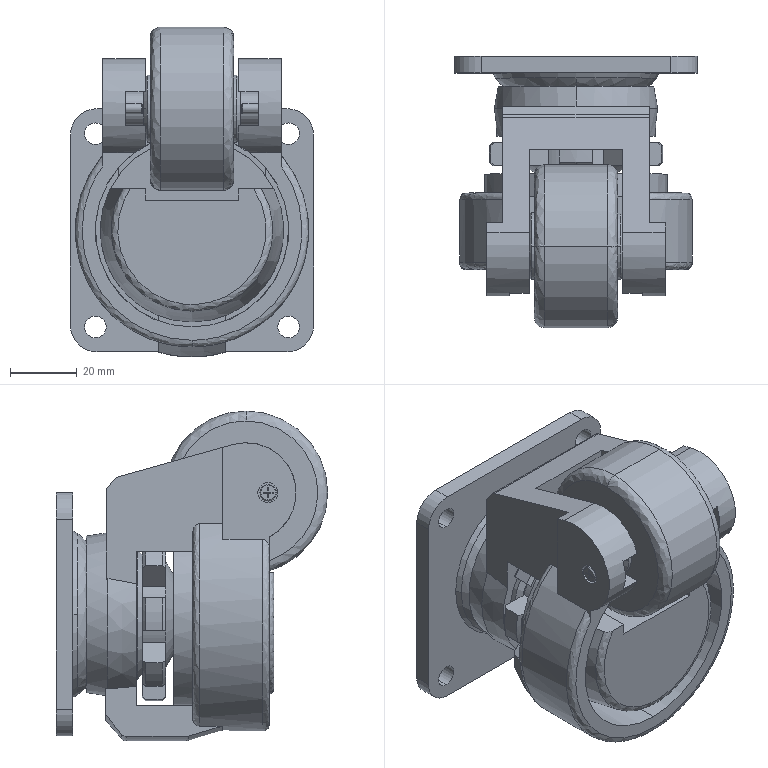Part | STEP file | CGR51-60-U Fuma caster | 4 solids | 294 faces | box 73 x 81.5 x 99 mm | volume 226029 mm3 | plane 128 | cylinder 82 | cone 69 | spline 15 | commonest cylinder face diameters 52 x9 6.5 x8 10 x8 35 x8 3 x6 5 x4